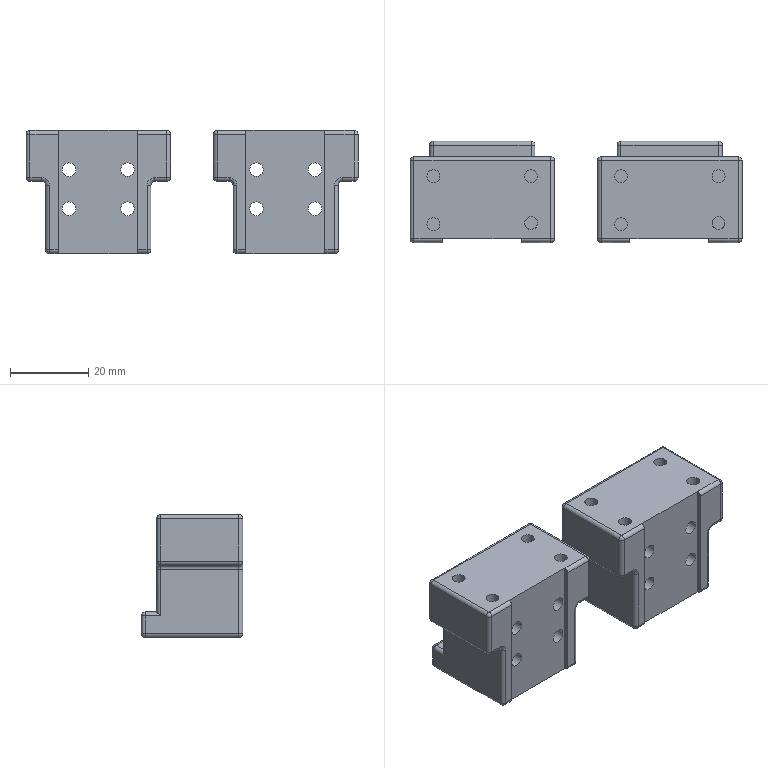Part | 2 solids | 186 faces | box 85 x 26 x 31.5 mm | volume 38654 mm3 | cylinder 90 | plane 52 | sphere 28 | torus 8 | cone 8 | commonest cylinder face diameters 2 x62 3.3 x8 3.5 x8 6 x8 1.6 x4